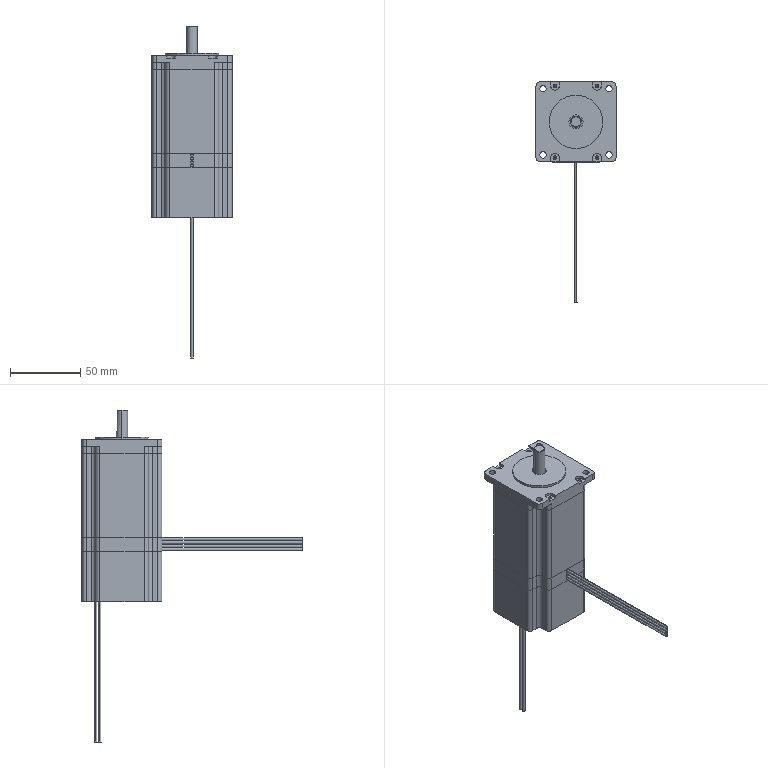Part | STEP file | Leadshine 57HSB21A (with brake) | 10 solids | 201 faces | box 57.15 x 157.15 x 237 mm | volume 340795 mm3 | cylinder 92 | plane 90 | cone 19 | commonest cylinder face diameters 6 x56 1.898 x8 2.5 x8 4.5 x8 2 x4 8 x2